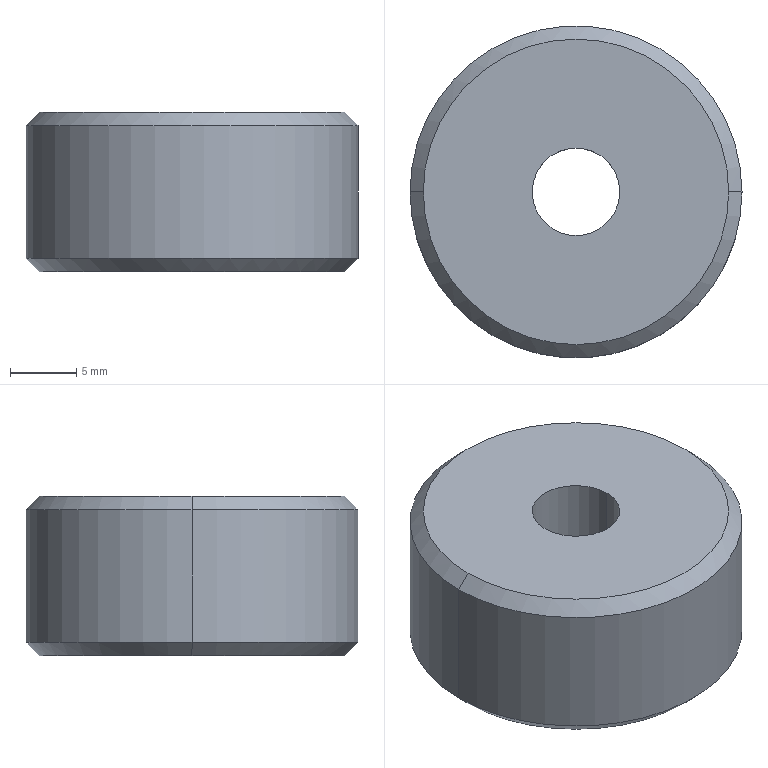Part | STEP file | 1 solid | 13 faces | box 25 x 25 x 12 mm | volume 5014 mm3 | cylinder 6 | cone 4 | plane 3 | commonest cylinder face diameters 6.6 x2 11 x2 25 x2
STEP:
#1=CARTESIAN_POINT('',(0.,0.,0.));
#2=DIRECTION('',(0.,0.,1.));
#3=DIRECTION('',(1.,0.,0.));
#4=AXIS2_PLACEMENT_3D('',#1,#2,#3);
#5=CARTESIAN_POINT('',(-11.5,0.,0.));
#6=VERTEX_POINT('',#5);
#7=CARTESIAN_POINT('',(11.5,0.,0.));
#8=VERTEX_POINT('',#7);
#9=CARTESIAN_POINT('',(0.,0.,0.));
#10=DIRECTION('',(0.,0.,-1.));
#11=DIRECTION('',(1.,0.,0.));
#12=AXIS2_PLACEMENT_3D('',#9,#10,#11);
#13=CIRCLE('',#12,11.5);
#14=CARTESIAN_POINT('',(0.,0.,1.));
#15=DIRECTION('',(0.,0.,1.));
#16=DIRECTION('',(1.,0.,0.));
#17=AXIS2_PLACEMENT_3D('',#14,#15,#16);
#18=CONICAL_SURFACE('',#17,12.5,0.7854);
#19=CARTESIAN_POINT('',(6.283,-1.));
#20=DIRECTION('',(-1.,0.));
#21=VECTOR('',#20,1.);
#22=LINE('',#19,#21);
#23=(GEOMETRIC_REPRESENTATION_CONTEXT(2)PARAMETRIC_REPRESENTATION_CONTEXT()REPRESENTATION_CONTEXT('',''));
#24=DEFINITIONAL_REPRESENTATION('',(#22),#23);
#25=PCURVE('',#18,#24);
#26=CARTESIAN_POINT('',(0.,0.,0.));
#27=DIRECTION('',(0.,0.,1.));
#28=DIRECTION('',(1.,0.,0.));
#29=AXIS2_PLACEMENT_3D('',#26,#27,#28);
#30=PLANE('',#29);
#31=CARTESIAN_POINT('',(11.5,0.));
#32=CARTESIAN_POINT('',(11.5,-19.919));
#33=CARTESIAN_POINT('',(-5.75,-9.959));
#34=CARTESIAN_POINT('',(-23.,0.));
#35=CARTESIAN_POINT('',(-5.75,9.959));
#36=CARTESIAN_POINT('',(11.5,19.919));
#37=CARTESIAN_POINT('',(11.5,0.));
#38=(BOUNDED_CURVE()B_SPLINE_CURVE(2,(#31,#32,#33,#34,#35,#36,#37),.UNSPECIFIED.,.T.,.F.)B_SPLINE_CURVE_WITH_KNOTS((1,2,2,2,2,1),(-2.094,0.,2.094,4.189,6.283,8.378),.UNSPECIFIED.)CURVE()GEOMETRIC_REPRESENTATION_ITEM()RATIONAL_B_SPLINE_CURVE((1.,0.5,1.,0.5,1.,0.5,1.))REPRESENTATION_ITEM(''));
#39=(GEOMETRIC_REPRESENTATION_CONTEXT(2)PARAMETRIC_REPRESENTATION_CONTEXT()REPRESENTATION_CONTEXT('',''));
#40=DEFINITIONAL_REPRESENTATION('',(#38),#39);
#41=PCURVE('',#30,#40);
#42=SURFACE_CURVE('',#13,(#25,#41),.PCURVE_S1.);
#43=EDGE_CURVE('',#6,#8,#42,.T.);
#44=ORIENTED_EDGE('',*,*,#43,.F.);
#45=CARTESIAN_POINT('',(-12.5,0.,1.));
#46=VERTEX_POINT('',#45);
#47=CARTESIAN_POINT('',(-12.5,0.,1.));
#48=DIRECTION('',(-0.7071,0.,0.7071));
#49=VECTOR('',#48,1.);
#50=LINE('',#47,#49);
#51=CARTESIAN_POINT('',(3.142,0.));
#52=DIRECTION('',(0.,1.));
#53=VECTOR('',#52,1.);
#54=LINE('',#51,#53);
#55=(GEOMETRIC_REPRESENTATION_CONTEXT(2)PARAMETRIC_REPRESENTATION_CONTEXT()REPRESENTATION_CONTEXT('',''));
#56=DEFINITIONAL_REPRESENTATION('',(#54),#55);
#57=PCURVE('',#18,#56);
#58=CARTESIAN_POINT('',(0.,0.,1.));
#59=DIRECTION('',(0.,0.,1.));
#60=DIRECTION('',(1.,0.,0.));
#61=AXIS2_PLACEMENT_3D('',#58,#59,#60);
#62=CONICAL_SURFACE('',#61,12.5,0.7854);
#63=CARTESIAN_POINT('',(3.142,0.));
#64=DIRECTION('',(0.,1.));
#65=VECTOR('',#64,1.);
#66=LINE('',#63,#65);
#67=(GEOMETRIC_REPRESENTATION_CONTEXT(2)PARAMETRIC_REPRESENTATION_CONTEXT()REPRESENTATION_CONTEXT('',''));
#68=DEFINITIONAL_REPRESENTATION('',(#66),#67);
#69=PCURVE('',#62,#68);
#70=SURFACE_CURVE('',#50,(#57,#69),.PCURVE_S1.);
#71=EDGE_CURVE('',#6,#46,#70,.T.);
#72=ORIENTED_EDGE('',*,*,#71,.T.);
#73=CARTESIAN_POINT('',(12.5,0.,1.));
#74=VERTEX_POINT('',#73);
#75=CARTESIAN_POINT('',(0.,0.,1.));
#76=DIRECTION('',(0.,0.,1.));
#77=DIRECTION('',(1.,0.,0.));
#78=AXIS2_PLACEMENT_3D('',#75,#76,#77);
#79=CIRCLE('',#78,12.5);
#80=CARTESIAN_POINT('',(0.,0.));
#81=DIRECTION('',(1.,0.));
#82=VECTOR('',#81,1.);
#83=LINE('',#80,#82);
#84=(GEOMETRIC_REPRESENTATION_CONTEXT(2)PARAMETRIC_REPRESENTATION_CONTEXT()REPRESENTATION_CONTEXT('',''));
#85=DEFINITIONAL_REPRESENTATION('',(#83),#84);
#86=PCURVE('',#18,#85);
#87=CARTESIAN_POINT('',(0.,0.,12.));
#88=DIRECTION('',(0.,0.,-1.));
#89=DIRECTION('',(-1.,0.,0.));
#90=AXIS2_PLACEMENT_3D('',#87,#88,#89);
#91=CYLINDRICAL_SURFACE('',#90,12.5);
#92=CARTESIAN_POINT('',(3.142,11.));
#93=DIRECTION('',(-1.,0.));
#94=VECTOR('',#93,1.);
#95=LINE('',#92,#94);
#96=(GEOMETRIC_REPRESENTATION_CONTEXT(2)PARAMETRIC_REPRESENTATION_CONTEXT()REPRESENTATION_CONTEXT('',''));
#97=DEFINITIONAL_REPRESENTATION('',(#95),#96);
#98=PCURVE('',#91,#97);
#99=SURFACE_CURVE('',#79,(#86,#98),.PCURVE_S1.);
#100=EDGE_CURVE('',#74,#46,#99,.T.);
#101=ORIENTED_EDGE('',*,*,#100,.F.);
#102=CARTESIAN_POINT('',(12.5,0.,1.));
#103=DIRECTION('',(0.7071,0.,0.7071));
#104=VECTOR('',#103,1.);
#105=LINE('',#102,#104);
#106=CARTESIAN_POINT('',(0.,0.));
#107=DIRECTION('',(0.,1.));
#108=VECTOR('',#107,1.);
#109=LINE('',#106,#108);
#110=(GEOMETRIC_REPRESENTATION_CONTEXT(2)PARAMETRIC_REPRESENTATION_CONTEXT()REPRESENTATION_CONTEXT('',''));
#111=DEFINITIONAL_REPRESENTATION('',(#109),#110);
#112=PCURVE('',#18,#111);
#113=CARTESIAN_POINT('',(6.283,0.));
#114=DIRECTION('',(0.,1.));
#115=VECTOR('',#114,1.);
#116=LINE('',#113,#115);
#117=(GEOMETRIC_REPRESENTATION_CONTEXT(2)PARAMETRIC_REPRESENTATION_CONTEXT()REPRESENTATION_CONTEXT('',''));
#118=DEFINITIONAL_REPRESENTATION('',(#116),#117);
#119=PCURVE('',#62,#118);
#120=SURFACE_CURVE('',#105,(#112,#119),.PCURVE_S1.);
#121=EDGE_CURVE('',#8,#74,#120,.T.);
#122=ORIENTED_EDGE('',*,*,#121,.F.);
#123=EDGE_LOOP('',(#44,#72,#101,#122));
#124=FACE_BOUND('',#123,.T.);
#125=ADVANCED_FACE('',(#124),#18,.T.);
#126=CARTESIAN_POINT('',(11.5,0.,12.));
#127=VERTEX_POINT('',#126);
#128=CARTESIAN_POINT('',(-11.5,0.,12.));
#129=VERTEX_POINT('',#128);
#130=CARTESIAN_POINT('',(0.,0.,12.));
#131=DIRECTION('',(0.,0.,1.));
#132=DIRECTION('',(1.,0.,0.));
#133=AXIS2_PLACEMENT_3D('',#130,#131,#132);
#134=CIRCLE('',#133,11.5);
#135=CARTESIAN_POINT('',(0.,0.,12.));
#136=DIRECTION('',(0.,0.,-1.));
#137=DIRECTION('',(-1.,0.,0.));
#138=AXIS2_PLACEMENT_3D('',#135,#136,#137);
#139=CONICAL_SURFACE('',#138,11.5,0.7854);
#140=CARTESIAN_POINT('',(3.142,0.));
#141=DIRECTION('',(-1.,0.));
#142=VECTOR('',#141,1.);
#143=LINE('',#140,#142);
#144=(GEOMETRIC_REPRESENTATION_CONTEXT(2)PARAMETRIC_REPRESENTATION_CONTEXT()REPRESENTATION_CONTEXT('',''));
#145=DEFINITIONAL_REPRESENTATION('',(#143),#144);
#146=PCURVE('',#139,#145);
#147=CARTESIAN_POINT('',(0.,0.,12.));
#148=DIRECTION('',(0.,0.,1.));
#149=DIRECTION('',(1.,0.,0.));
#150=AXIS2_PLACEMENT_3D('',#147,#148,#149);
#151=PLANE('',#150);
#152=CARTESIAN_POINT('',(0.,0.));
#153=DIRECTION('',(1.,0.));
#154=AXIS2_PLACEMENT_2D('',#152,#153);
#155=CIRCLE('',#154,11.5);
#156=(GEOMETRIC_REPRESENTATION_CONTEXT(2)PARAMETRIC_REPRESENTATION_CONTEXT()REPRESENTATION_CONTEXT('',''));
#157=DEFINITIONAL_REPRESENTATION('',(#155),#156);
#158=PCURVE('',#151,#157);
#159=SURFACE_CURVE('',#134,(#146,#158),.PCURVE_S1.);
#160=EDGE_CURVE('',#127,#129,#159,.T.);
#161=ORIENTED_EDGE('',*,*,#160,.F.);
#162=CARTESIAN_POINT('',(12.5,0.,11.));
#163=VERTEX_POINT('',#162);
#164=CARTESIAN_POINT('',(11.5,0.,12.));
#165=DIRECTION('',(0.7071,0.,-0.7071));
#166=VECTOR('',#165,1.);
#167=LINE('',#164,#166);
#168=CARTESIAN_POINT('',(3.142,0.));
#169=DIRECTION('',(0.,1.));
#170=VECTOR('',#169,1.);
#171=LINE('',#168,#170);
#172=(GEOMETRIC_REPRESENTATION_CONTEXT(2)PARAMETRIC_REPRESENTATION_CONTEXT()REPRESENTATION_CONTEXT('',''));
#173=DEFINITIONAL_REPRESENTATION('',(#171),#172);
#174=PCURVE('',#139,#173);
#175=CARTESIAN_POINT('',(0.,0.,12.));
#176=DIRECTION('',(0.,0.,-1.));
#177=DIRECTION('',(-1.,0.,0.));
#178=AXIS2_PLACEMENT_3D('',#175,#176,#177);
#179=CONICAL_SURFACE('',#178,11.5,0.7854);
#180=CARTESIAN_POINT('',(3.142,0.));
#181=DIRECTION('',(0.,1.));
#182=VECTOR('',#181,1.);
#183=LINE('',#180,#182);
#184=(GEOMETRIC_REPRESENTATION_CONTEXT(2)PARAMETRIC_REPRESENTATION_CONTEXT()REPRESENTATION_CONTEXT('',''));
#185=DEFINITIONAL_REPRESENTATION('',(#183),#184);
#186=PCURVE('',#179,#185);
#187=SURFACE_CURVE('',#167,(#174,#186),.PCURVE_S1.);
#188=EDGE_CURVE('',#127,#163,#187,.T.);
#189=ORIENTED_EDGE('',*,*,#188,.T.);
#190=CARTESIAN_POINT('',(-12.5,0.,11.));
#191=VERTEX_POINT('',#190);
#192=CARTESIAN_POINT('',(0.,0.,11.));
#193=DIRECTION('',(0.,0.,-1.));
#194=DIRECTION('',(1.,0.,0.));
#195=AXIS2_PLACEMENT_3D('',#192,#193,#194);
#196=CIRCLE('',#195,12.5);
#197=CARTESIAN_POINT('',(-3.142,1.));
#198=DIRECTION('',(1.,0.));
#199=VECTOR('',#198,1.);
#200=LINE('',#197,#199);
#201=(GEOMETRIC_REPRESENTATION_CONTEXT(2)PARAMETRIC_REPRESENTATION_CONTEXT()REPRESENTATION_CONTEXT('',''));
#202=DEFINITIONAL_REPRESENTATION('',(#200),#201);
#203=PCURVE('',#139,#202);
#204=CARTESIAN_POINT('',(-3.142,1.));
#205=DIRECTION('',(1.,0.));
#206=VECTOR('',#205,1.);
#207=LINE('',#204,#206);
#208=(GEOMETRIC_REPRESENTATION_CONTEXT(2)PARAMETRIC_REPRESENTATION_CONTEXT()REPRESENTATION_CONTEXT('',''));
#209=DEFINITIONAL_REPRESENTATION('',(#207),#208);
#210=PCURVE('',#91,#209);
#211=SURFACE_CURVE('',#196,(#203,#210),.PCURVE_S1.);
#212=EDGE_CURVE('',#191,#163,#211,.T.);
#213=ORIENTED_EDGE('',*,*,#212,.F.);
#214=CARTESIAN_POINT('',(-11.5,0.,12.));
#215=DIRECTION('',(-0.7071,0.,-0.7071));
#216=VECTOR('',#215,1.);
#217=LINE('',#214,#216);
#218=CARTESIAN_POINT('',(0.,0.));
#219=DIRECTION('',(0.,1.));
#220=VECTOR('',#219,1.);
#221=LINE('',#218,#220);
#222=(GEOMETRIC_REPRESENTATION_CONTEXT(2)PARAMETRIC_REPRESENTATION_CONTEXT()REPRESENTATION_CONTEXT('',''));
#223=DEFINITIONAL_REPRESENTATION('',(#221),#222);
#224=PCURVE('',#139,#223);
#225=CARTESIAN_POINT('',(6.283,0.));
#226=DIRECTION('',(0.,1.));
#227=VECTOR('',#226,1.);
#228=LINE('',#225,#227);
#229=(GEOMETRIC_REPRESENTATION_CONTEXT(2)PARAMETRIC_REPRESENTATION_CONTEXT()REPRESENTATION_CONTEXT('',''));
#230=DEFINITIONAL_REPRESENTATION('',(#228),#229);
#231=PCURVE('',#179,#230);
#232=SURFACE_CURVE('',#217,(#224,#231),.PCURVE_S1.);
#233=EDGE_CURVE('',#129,#191,#232,.T.);
#234=ORIENTED_EDGE('',*,*,#233,.F.);
#235=EDGE_LOOP('',(#161,#189,#213,#234));
#236=FACE_BOUND('',#235,.T.);
#237=ADVANCED_FACE('',(#236),#139,.T.);
#238=CARTESIAN_POINT('',(-5.5,0.,6.4));
#239=VERTEX_POINT('',#238);
#240=CARTESIAN_POINT('',(-5.5,0.,0.));
#241=VERTEX_POINT('',#240);
#242=CARTESIAN_POINT('',(-5.5,0.,0.));
#243=DIRECTION('',(0.,0.,-1.));
#244=VECTOR('',#243,1.);
#245=LINE('',#242,#244);
#246=CARTESIAN_POINT('',(0.,0.,0.));
#247=DIRECTION('',(0.,0.,-1.));
#248=DIRECTION('',(-1.,0.,0.));
#249=AXIS2_PLACEMENT_3D('',#246,#247,#248);
#250=CYLINDRICAL_SURFACE('',#249,5.5);
#251=CARTESIAN_POINT('',(6.283,0.));
#252=DIRECTION('',(0.,1.));
#253=VECTOR('',#252,1.);
#254=LINE('',#251,#253);
#255=(GEOMETRIC_REPRESENTATION_CONTEXT(2)PARAMETRIC_REPRESENTATION_CONTEXT()REPRESENTATION_CONTEXT('',''));
#256=DEFINITIONAL_REPRESENTATION('',(#254),#255);
#257=PCURVE('',#250,#256);
#258=CARTESIAN_POINT('',(0.,0.,0.));
#259=DIRECTION('',(0.,0.,-1.));
#260=DIRECTION('',(-1.,0.,0.));
#261=AXIS2_PLACEMENT_3D('',#258,#259,#260);
#262=CYLINDRICAL_SURFACE('',#261,5.5);
#263=CARTESIAN_POINT('',(0.,0.));
#264=DIRECTION('',(0.,1.));
#265=VECTOR('',#264,1.);
#266=LINE('',#263,#265);
#267=(GEOMETRIC_REPRESENTATION_CONTEXT(2)PARAMETRIC_REPRESENTATION_CONTEXT()REPRESENTATION_CONTEXT('',''));
#268=DEFINITIONAL_REPRESENTATION('',(#266),#267);
#269=PCURVE('',#262,#268);
#270=SURFACE_CURVE('',#245,(#257,#269),.PCURVE_S1.);
#271=EDGE_CURVE('',#239,#241,#270,.T.);
#272=ORIENTED_EDGE('',*,*,#271,.T.);
#273=CARTESIAN_POINT('',(5.5,0.,0.));
#274=VERTEX_POINT('',#273);
#275=CARTESIAN_POINT('',(0.,0.,0.));
#276=DIRECTION('',(0.,0.,-1.));
#277=DIRECTION('',(-1.,0.,0.));
#278=AXIS2_PLACEMENT_3D('',#275,#276,#277);
#279=CIRCLE('',#278,5.5);
#280=CARTESIAN_POINT('',(0.,0.));
#281=DIRECTION('',(1.,0.));
#282=VECTOR('',#281,1.);
#283=LINE('',#280,#282);
#284=(GEOMETRIC_REPRESENTATION_CONTEXT(2)PARAMETRIC_REPRESENTATION_CONTEXT()REPRESENTATION_CONTEXT('',''));
#285=DEFINITIONAL_REPRESENTATION('',(#283),#284);
#286=PCURVE('',#250,#285);
#287=CARTESIAN_POINT('',(-5.5,0.));
#288=CARTESIAN_POINT('',(-5.5,9.526));
#289=CARTESIAN_POINT('',(2.75,4.763));
#290=CARTESIAN_POINT('',(11.,0.));
#291=CARTESIAN_POINT('',(2.75,-4.763));
#292=CARTESIAN_POINT('',(-5.5,-9.526));
#293=CARTESIAN_POINT('',(-5.5,0.));
#294=(BOUNDED_CURVE()B_SPLINE_CURVE(2,(#287,#288,#289,#290,#291,#292,#293),.UNSPECIFIED.,.T.,.F.)B_SPLINE_CURVE_WITH_KNOTS((1,2,2,2,2,1),(-2.094,0.,2.094,4.189,6.283,8.378),.UNSPECIFIED.)CURVE()GEOMETRIC_REPRESENTATION_ITEM()RATIONAL_B_SPLINE_CURVE((1.,0.5,1.,0.5,1.,0.5,1.))REPRESENTATION_ITEM(''));
#295=(GEOMETRIC_REPRESENTATION_CONTEXT(2)PARAMETRIC_REPRESENTATION_CONTEXT()REPRESENTATION_CONTEXT('',''));
#296=DEFINITIONAL_REPRESENTATION('',(#294),#295);
#297=PCURVE('',#30,#296);
#298=SURFACE_CURVE('',#279,(#286,#297),.PCURVE_S1.);
#299=EDGE_CURVE('',#274,#241,#298,.T.);
#300=ORIENTED_EDGE('',*,*,#299,.F.);
#301=CARTESIAN_POINT('',(5.5,0.,6.4));
#302=VERTEX_POINT('',#301);
#303=CARTESIAN_POINT('',(5.5,0.,0.));
#304=DIRECTION('',(0.,0.,-1.));
#305=VECTOR('',#304,1.);
#306=LINE('',#303,#305);
#307=CARTESIAN_POINT('',(3.142,0.));
#308=DIRECTION('',(0.,1.));
#309=VECTOR('',#308,1.);
#310=LINE('',#307,#309);
#311=(GEOMETRIC_REPRESENTATION_CONTEXT(2)PARAMETRIC_REPRESENTATION_CONTEXT()REPRESENTATION_CONTEXT('',''));
#312=DEFINITIONAL_REPRESENTATION('',(#310),#311);
#313=PCURVE('',#250,#312);
#314=CARTESIAN_POINT('',(3.142,0.));
#315=DIRECTION('',(0.,1.));
#316=VECTOR('',#315,1.);
#317=LINE('',#314,#316);
#318=(GEOMETRIC_REPRESENTATION_CONTEXT(2)PARAMETRIC_REPRESENTATION_CONTEXT()REPRESENTATION_CONTEXT('',''));
#319=DEFINITIONAL_REPRESENTATION('',(#317),#318);
#320=PCURVE('',#262,#319);
#321=SURFACE_CURVE('',#306,(#313,#320),.PCURVE_S1.);
#322=EDGE_CURVE('',#302,#274,#321,.T.);
#323=ORIENTED_EDGE('',*,*,#322,.F.);
#324=CARTESIAN_POINT('',(0.,0.,6.4));
#325=DIRECTION('',(0.,0.,-1.));
#326=DIRECTION('',(-1.,0.,0.));
#327=AXIS2_PLACEMENT_3D('',#324,#325,#326);
#328=CIRCLE('',#327,5.5);
#329=CARTESIAN_POINT('',(0.,-6.4));
#330=DIRECTION('',(1.,0.));
#331=VECTOR('',#330,1.);
#332=LINE('',#329,#331);
#333=(GEOMETRIC_REPRESENTATION_CONTEXT(2)PARAMETRIC_REPRESENTATION_CONTEXT()REPRESENTATION_CONTEXT('',''));
#334=DEFINITIONAL_REPRESENTATION('',(#332),#333);
#335=PCURVE('',#250,#334);
#336=CARTESIAN_POINT('',(3.3,0.,6.4));
#337=DIRECTION('',(0.,0.,1.));
#338=DIRECTION('',(1.,0.,0.));
#339=AXIS2_PLACEMENT_3D('',#336,#337,#338);
#340=PLANE('',#339);
#341=CARTESIAN_POINT('',(-8.8,0.));
#342=CARTESIAN_POINT('',(-8.8,9.526));
#343=CARTESIAN_POINT('',(-0.55,4.763));
#344=CARTESIAN_POINT('',(7.7,0.));
#345=CARTESIAN_POINT('',(-0.55,-4.763));
#346=CARTESIAN_POINT('',(-8.8,-9.526));
#347=CARTESIAN_POINT('',(-8.8,0.));
#348=(BOUNDED_CURVE()B_SPLINE_CURVE(2,(#341,#342,#343,#344,#345,#346,#347),.UNSPECIFIED.,.T.,.F.)B_SPLINE_CURVE_WITH_KNOTS((1,2,2,2,2,1),(-2.094,0.,2.094,4.189,6.283,8.378),.UNSPECIFIED.)CURVE()GEOMETRIC_REPRESENTATION_ITEM()RATIONAL_B_SPLINE_CURVE((1.,0.5,1.,0.5,1.,0.5,1.))REPRESENTATION_ITEM(''));
#349=(GEOMETRIC_REPRESENTATION_CONTEXT(2)PARAMETRIC_REPRESENTATION_CONTEXT()REPRESENTATION_CONTEXT('',''));
#350=DEFINITIONAL_REPRESENTATION('',(#348),#349);
#351=PCURVE('',#340,#350);
#352=SURFACE_CURVE('',#328,(#335,#351),.PCURVE_S1.);
#353=EDGE_CURVE('',#302,#239,#352,.T.);
#354=ORIENTED_EDGE('',*,*,#353,.T.);
#355=EDGE_LOOP('',(#272,#300,#323,#354));
#356=FACE_BOUND('',#355,.F.);
#357=ADVANCED_FACE('',(#356),#250,.F.);
#358=CARTESIAN_POINT('',(-3.3,0.,12.));
#359=VERTEX_POINT('',#358);
#360=CARTESIAN_POINT('',(-3.3,0.,6.4));
#361=VERTEX_POINT('',#360);
#362=CARTESIAN_POINT('',(-3.3,0.,0.));
#363=DIRECTION('',(0.,0.,-1.));
#364=VECTOR('',#363,1.);
#365=LINE('',#362,#364);
#366=CARTESIAN_POINT('',(0.,0.,0.));
#367=DIRECTION('',(0.,0.,-1.));
#368=DIRECTION('',(-1.,0.,0.));
#369=AXIS2_PLACEMENT_3D('',#366,#367,#368);
#370=CYLINDRICAL_SURFACE('',#369,3.3);
#371=CARTESIAN_POINT('',(6.283,0.));
#372=DIRECTION('',(0.,1.));
#373=VECTOR('',#372,1.);
#374=LINE('',#371,#373);
#375=(GEOMETRIC_REPRESENTATION_CONTEXT(2)PARAMETRIC_REPRESENTATION_CONTEXT()REPRESENTATION_CONTEXT('',''));
#376=DEFINITIONAL_REPRESENTATION('',(#374),#375);
#377=PCURVE('',#370,#376);
#378=CARTESIAN_POINT('',(0.,0.,0.));
#379=DIRECTION('',(0.,0.,-1.));
#380=DIRECTION('',(-1.,0.,0.));
#381=AXIS2_PLACEMENT_3D('',#378,#379,#380);
#382=CYLINDRICAL_SURFACE('',#381,3.3);
#383=CARTESIAN_POINT('',(0.,0.));
#384=DIRECTION('',(0.,1.));
#385=VECTOR('',#384,1.);
#386=LINE('',#383,#385);
#387=(GEOMETRIC_REPRESENTATION_CONTEXT(2)PARAMETRIC_REPRESENTATION_CONTEXT()REPRESENTATION_CONTEXT('',''));
#388=DEFINITIONAL_REPRESENTATION('',(#386),#387);
#389=PCURVE('',#382,#388);
#390=SURFACE_CURVE('',#365,(#377,#389),.PCURVE_S1.);
#391=EDGE_CURVE('',#359,#361,#390,.T.);
#392=ORIENTED_EDGE('',*,*,#391,.T.);
#393=CARTESIAN_POINT('',(3.3,0.,6.4));
#394=VERTEX_POINT('',#393);
#395=CARTESIAN_POINT('',(0.,0.,6.4));
#396=DIRECTION('',(0.,0.,-1.));
#397=DIRECTION('',(-1.,0.,0.));
#398=AXIS2_PLACEMENT_3D('',#395,#396,#397);
#399=CIRCLE('',#398,3.3);
#400=CARTESIAN_POINT('',(0.,-6.4));
#401=DIRECTION('',(1.,0.));
#402=VECTOR('',#401,1.);
#403=LINE('',#400,#402);
#404=(GEOMETRIC_REPRESENTATION_CONTEXT(2)PARAMETRIC_REPRESENTATION_CONTEXT()REPRESENTATION_CONTEXT('',''));
#405=DEFINITIONAL_REPRESENTATION('',(#403),#404);
#406=PCURVE('',#370,#405);
#407=CARTESIAN_POINT('',(-6.6,0.));
#408=CARTESIAN_POINT('',(-6.6,5.716));
#409=CARTESIAN_POINT('',(-1.65,2.858));
#410=CARTESIAN_POINT('',(3.3,0.));
#411=CARTESIAN_POINT('',(-1.65,-2.858));
#412=CARTESIAN_POINT('',(-6.6,-5.716));
#413=CARTESIAN_POINT('',(-6.6,0.));
#414=(BOUNDED_CURVE()B_SPLINE_CURVE(2,(#407,#408,#409,#410,#411,#412,#413),.UNSPECIFIED.,.T.,.F.)B_SPLINE_CURVE_WITH_KNOTS((1,2,2,2,2,1),(-2.094,0.,2.094,4.189,6.283,8.378),.UNSPECIFIED.)CURVE()GEOMETRIC_REPRESENTATION_ITEM()RATIONAL_B_SPLINE_CURVE((1.,0.5,1.,0.5,1.,0.5,1.))REPRESENTATION_ITEM(''));
#415=(GEOMETRIC_REPRESENTATION_CONTEXT(2)PARAMETRIC_REPRESENTATION_CONTEXT()REPRESENTATION_CONTEXT('',''));
#416=DEFINITIONAL_REPRESENTATION('',(#414),#415);
#417=PCURVE('',#340,#416);
#418=SURFACE_CURVE('',#399,(#406,#417),.PCURVE_S1.);
#419=EDGE_CURVE('',#394,#361,#418,.T.);
#420=ORIENTED_EDGE('',*,*,#419,.F.);
#421=CARTESIAN_POINT('',(3.3,0.,12.));
#422=VERTEX_POINT('',#421);
#423=CARTESIAN_POINT('',(3.3,0.,0.));
#424=DIRECTION('',(0.,0.,-1.));
#425=VECTOR('',#424,1.);
#426=LINE('',#423,#425);
#427=CARTESIAN_POINT('',(3.142,0.));
#428=DIRECTION('',(0.,1.));
#429=VECTOR('',#428,1.);
#430=LINE('',#427,#429);
#431=(GEOMETRIC_REPRESENTATION_CONTEXT(2)PARAMETRIC_REPRESENTATION_CONTEXT()REPRESENTATION_CONTEXT('',''));
#432=DEFINITIONAL_REPRESENTATION('',(#430),#431);
#433=PCURVE('',#370,#432);
#434=CARTESIAN_POINT('',(3.142,0.));
#435=DIRECTION('',(0.,1.));
#436=VECTOR('',#435,1.);
#437=LINE('',#434,#436);
#438=(GEOMETRIC_REPRESENTATION_CONTEXT(2)PARAMETRIC_REPRESENTATION_CONTEXT()REPRESENTATION_CONTEXT('',''));
#439=DEFINITIONAL_REPRESENTATION('',(#437),#438);
#440=PCURVE('',#382,#439);
#441=SURFACE_CURVE('',#426,(#433,#440),.PCURVE_S1.);
#442=EDGE_CURVE('',#422,#394,#441,.T.);
#443=ORIENTED_EDGE('',*,*,#442,.F.);
#444=CARTESIAN_POINT('',(0.,0.,12.));
#445=DIRECTION('',(0.,0.,-1.));
#446=DIRECTION('',(-1.,0.,0.));
#447=AXIS2_PLACEMENT_3D('',#444,#445,#446);
#448=CIRCLE('',#447,3.3);
#449=CARTESIAN_POINT('',(0.,-12.));
#450=DIRECTION('',(1.,0.));
#451=VECTOR('',#450,1.);
#452=LINE('',#449,#451);
#453=(GEOMETRIC_REPRESENTATION_CONTEXT(2)PARAMETRIC_REPRESENTATION_CONTEXT()REPRESENTATION_CONTEXT('',''));
#454=DEFINITIONAL_REPRESENTATION('',(#452),#453);
#455=PCURVE('',#370,#454);
#456=CARTESIAN_POINT('',(-3.3,0.));
#457=CARTESIAN_POINT('',(-3.3,5.716));
#458=CARTESIAN_POINT('',(1.65,2.858));
#459=CARTESIAN_POINT('',(6.6,0.));
#460=CARTESIAN_POINT('',(1.65,-2.858));
#461=CARTESIAN_POINT('',(-3.3,-5.716));
#462=CARTESIAN_POINT('',(-3.3,0.));
#463=(BOUNDED_CURVE()B_SPLINE_CURVE(2,(#456,#457,#458,#459,#460,#461,#462),.UNSPECIFIED.,.T.,.F.)B_SPLINE_CURVE_WITH_KNOTS((1,2,2,2,2,1),(-2.094,0.,2.094,4.189,6.283,8.378),.UNSPECIFIED.)CURVE()GEOMETRIC_REPRESENTATION_ITEM()RATIONAL_B_SPLINE_CURVE((1.,0.5,1.,0.5,1.,0.5,1.))REPRESENTATION_ITEM(''));
#464=(GEOMETRIC_REPRESENTATION_CONTEXT(2)PARAMETRIC_REPRESENTATION_CONTEXT()REPRESENTATION_CONTEXT('',''));
#465=DEFINITIONAL_REPRESENTATION('',(#463),#464);
#466=PCURVE('',#151,#465);
#467=SURFACE_CURVE('',#448,(#455,#466),.PCURVE_S1.);
#468=EDGE_CURVE('',#422,#359,#467,.T.);
#469=ORIENTED_EDGE('',*,*,#468,.T.);
#470=EDGE_LOOP('',(#392,#420,#443,#469));
#471=FACE_BOUND('',#470,.F.);
#472=ADVANCED_FACE('',(#471),#370,.F.);
#473=ORIENTED_EDGE('',*,*,#212,.T.);
#474=CARTESIAN_POINT('',(12.5,0.,12.));
#475=DIRECTION('',(0.,0.,-1.));
#476=VECTOR('',#475,1.);
#477=LINE('',#474,#476);
#478=CARTESIAN_POINT('',(3.142,0.));
#479=DIRECTION('',(0.,1.));
#480=VECTOR('',#479,1.);
#481=LINE('',#478,#480);
#482=(GEOMETRIC_REPRESENTATION_CONTEXT(2)PARAMETRIC_REPRESENTATION_CONTEXT()REPRESENTATION_CONTEXT('',''));
#483=DEFINITIONAL_REPRESENTATION('',(#481),#482);
#484=PCURVE('',#91,#483);
#485=CARTESIAN_POINT('',(0.,0.,12.));
#486=DIRECTION('',(0.,0.,-1.));
#487=DIRECTION('',(-1.,0.,0.));
#488=AXIS2_PLACEMENT_3D('',#485,#486,#487);
#489=CYLINDRICAL_SURFACE('',#488,12.5);
#490=CARTESIAN_POINT('',(3.142,0.));
#491=DIRECTION('',(0.,1.));
#492=VECTOR('',#491,1.);
#493=LINE('',#490,#492);
#494=(GEOMETRIC_REPRESENTATION_CONTEXT(2)PARAMETRIC_REPRESENTATION_CONTEXT()REPRESENTATION_CONTEXT('',''));
#495=DEFINITIONAL_REPRESENTATION('',(#493),#494);
#496=PCURVE('',#489,#495);
#497=SURFACE_CURVE('',#477,(#484,#496),.PCURVE_S1.);
#498=EDGE_CURVE('',#163,#74,#497,.T.);
#499=ORIENTED_EDGE('',*,*,#498,.T.);
#500=ORIENTED_EDGE('',*,*,#100,.T.);
#501=CARTESIAN_POINT('',(-12.5,0.,12.));
#502=DIRECTION('',(0.,0.,-1.));
#503=VECTOR('',#502,1.);
#504=LINE('',#501,#503);
#505=CARTESIAN_POINT('',(0.,0.));
#506=DIRECTION('',(0.,1.));
#507=VECTOR('',#506,1.);
#508=LINE('',#505,#507);
#509=(GEOMETRIC_REPRESENTATION_CONTEXT(2)PARAMETRIC_REPRESENTATION_CONTEXT()REPRESENTATION_CONTEXT('',''));
#510=DEFINITIONAL_REPRESENTATION('',(#508),#509);
#511=PCURVE('',#91,#510);
#512=CARTESIAN_POINT('',(6.283,0.));
#513=DIRECTION('',(0.,1.));
#514=VECTOR('',#513,1.);
#515=LINE('',#512,#514);
#516=(GEOMETRIC_REPRESENTATION_CONTEXT(2)PARAMETRIC_REPRESENTATION_CONTEXT()REPRESENTATION_CONTEXT('',''));
#517=DEFINITIONAL_REPRESENTATION('',(#515),#516);
#518=PCURVE('',#489,#517);
#519=SURFACE_CURVE('',#504,(#511,#518),.PCURVE_S1.);
#520=EDGE_CURVE('',#191,#46,#519,.T.);
#521=ORIENTED_EDGE('',*,*,#520,.F.);
#522=EDGE_LOOP('',(#473,#499,#500,#521));
#523=FACE_BOUND('',#522,.T.);
#524=ADVANCED_FACE('',(#523),#91,.T.);
#525=ORIENTED_EDGE('',*,*,#498,.F.);
#526=CARTESIAN_POINT('',(0.,0.,11.));
#527=DIRECTION('',(0.,0.,-1.));
#528=DIRECTION('',(1.,0.,0.));
#529=AXIS2_PLACEMENT_3D('',#526,#527,#528);
#530=CIRCLE('',#529,12.5);
#531=CARTESIAN_POINT('',(3.142,1.));
#532=DIRECTION('',(1.,0.));
#533=VECTOR('',#532,1.);
#534=LINE('',#531,#533);
#535=(GEOMETRIC_REPRESENTATION_CONTEXT(2)PARAMETRIC_REPRESENTATION_CONTEXT()REPRESENTATION_CONTEXT('',''));
#536=DEFINITIONAL_REPRESENTATION('',(#534),#535);
#537=PCURVE('',#489,#536);
#538=CARTESIAN_POINT('',(3.142,1.));
#539=DIRECTION('',(1.,0.));
#540=VECTOR('',#539,1.);
#541=LINE('',#538,#540);
#542=(GEOMETRIC_REPRESENTATION_CONTEXT(2)PARAMETRIC_REPRESENTATION_CONTEXT()REPRESENTATION_CONTEXT('',''));
#543=DEFINITIONAL_REPRESENTATION('',(#541),#542);
#544=PCURVE('',#179,#543);
#545=SURFACE_CURVE('',#530,(#537,#544),.PCURVE_S1.);
#546=EDGE_CURVE('',#163,#191,#545,.T.);
#547=ORIENTED_EDGE('',*,*,#546,.T.);
#548=ORIENTED_EDGE('',*,*,#520,.T.);
#549=CARTESIAN_POINT('',(0.,0.,1.));
#550=DIRECTION('',(0.,0.,1.));
#551=DIRECTION('',(1.,0.,0.));
#552=AXIS2_PLACEMENT_3D('',#549,#550,#551);
#553=CIRCLE('',#552,12.5);
#554=CARTESIAN_POINT('',(9.425,11.));
#555=DIRECTION('',(-1.,0.));
#556=VECTOR('',#555,1.);
#557=LINE('',#554,#556);
#558=(GEOMETRIC_REPRESENTATION_CONTEXT(2)PARAMETRIC_REPRESENTATION_CONTEXT()REPRESENTATION_CONTEXT('',''));
#559=DEFINITIONAL_REPRESENTATION('',(#557),#558);
#560=PCURVE('',#489,#559);
#561=CARTESIAN_POINT('',(0.,0.));
#562=DIRECTION('',(1.,0.));
#563=VECTOR('',#562,1.);
#564=LINE('',#561,#563);
#565=(GEOMETRIC_REPRESENTATION_CONTEXT(2)PARAMETRIC_REPRESENTATION_CONTEXT()REPRESENTATION_CONTEXT('',''));
#566=DEFINITIONAL_REPRESENTATION('',(#564),#565);
#567=PCURVE('',#62,#566);
#568=SURFACE_CURVE('',#553,(#560,#567),.PCURVE_S1.);
#569=EDGE_CURVE('',#46,#74,#568,.T.);
#570=ORIENTED_EDGE('',*,*,#569,.T.);
#571=EDGE_LOOP('',(#525,#547,#548,#570));
#572=FACE_BOUND('',#571,.T.);
#573=ADVANCED_FACE('',(#572),#489,.T.);
#574=CARTESIAN_POINT('',(0.,0.,12.));
#575=DIRECTION('',(0.,0.,1.));
#576=DIRECTION('',(1.,0.,0.));
#577=AXIS2_PLACEMENT_3D('',#574,#575,#576);
#578=CIRCLE('',#577,11.5);
#579=CARTESIAN_POINT('',(0.,0.));
#580=DIRECTION('',(1.,0.));
#581=AXIS2_PLACEMENT_2D('',#579,#580);
#582=CIRCLE('',#581,11.5);
#583=(GEOMETRIC_REPRESENTATION_CONTEXT(2)PARAMETRIC_REPRESENTATION_CONTEXT()REPRESENTATION_CONTEXT('',''));
#584=DEFINITIONAL_REPRESENTATION('',(#582),#583);
#585=PCURVE('',#151,#584);
#586=CARTESIAN_POINT('',(9.425,0.));
#587=DIRECTION('',(-1.,0.));
#588=VECTOR('',#587,1.);
#589=LINE('',#586,#588);
#590=(GEOMETRIC_REPRESENTATION_CONTEXT(2)PARAMETRIC_REPRESENTATION_CONTEXT()REPRESENTATION_CONTEXT('',''));
#591=DEFINITIONAL_REPRESENTATION('',(#589),#590);
#592=PCURVE('',#179,#591);
#593=SURFACE_CURVE('',#578,(#585,#592),.PCURVE_S1.);
#594=EDGE_CURVE('',#129,#127,#593,.T.);
#595=ORIENTED_EDGE('',*,*,#594,.T.);
#596=ORIENTED_EDGE('',*,*,#160,.T.);
#597=EDGE_LOOP('',(#595,#596));
#598=FACE_BOUND('',#597,.T.);
#599=CARTESIAN_POINT('',(0.,0.,12.));
#600=DIRECTION('',(0.,0.,-1.));
#601=DIRECTION('',(-1.,0.,0.));
#602=AXIS2_PLACEMENT_3D('',#599,#600,#601);
#603=CIRCLE('',#602,3.3);
#604=CARTESIAN_POINT('',(-3.3,0.));
#605=CARTESIAN_POINT('',(-3.3,5.716));
#606=CARTESIAN_POINT('',(1.65,2.858));
#607=CARTESIAN_POINT('',(6.6,0.));
#608=CARTESIAN_POINT('',(1.65,-2.858));
#609=CARTESIAN_POINT('',(-3.3,-5.716));
#610=CARTESIAN_POINT('',(-3.3,0.));
#611=(BOUNDED_CURVE()B_SPLINE_CURVE(2,(#604,#605,#606,#607,#608,#609,#610),.UNSPECIFIED.,.T.,.F.)B_SPLINE_CURVE_WITH_KNOTS((1,2,2,2,2,1),(-2.094,0.,2.094,4.189,6.283,8.378),.UNSPECIFIED.)CURVE()GEOMETRIC_REPRESENTATION_ITEM()RATIONAL_B_SPLINE_CURVE((1.,0.5,1.,0.5,1.,0.5,1.))REPRESENTATION_ITEM(''));
#612=(GEOMETRIC_REPRESENTATION_CONTEXT(2)PARAMETRIC_REPRESENTATION_CONTEXT()REPRESENTATION_CONTEXT('',''));
#613=DEFINITIONAL_REPRESENTATION('',(#611),#612);
#614=PCURVE('',#151,#613);
#615=CARTESIAN_POINT('',(0.,-12.));
#616=DIRECTION('',(1.,0.));
#617=VECTOR('',#616,1.);
#618=LINE('',#615,#617);
#619=(GEOMETRIC_REPRESENTATION_CONTEXT(2)PARAMETRIC_REPRESENTATION_CONTEXT()REPRESENTATION_CONTEXT('',''));
#620=DEFINITIONAL_REPRESENTATION('',(#618),#619);
#621=PCURVE('',#382,#620);
#622=SURFACE_CURVE('',#603,(#614,#621),.PCURVE_S1.);
#623=EDGE_CURVE('',#359,#422,#622,.T.);
#624=ORIENTED_EDGE('',*,*,#623,.T.);
#625=ORIENTED_EDGE('',*,*,#468,.T.);
#626=EDGE_LOOP('',(#624,#625));
#627=FACE_BOUND('',#626,.T.);
#628=ADVANCED_FACE('',(#598,#627),#151,.T.);
#629=CARTESIAN_POINT('',(0.,0.,0.));
#630=DIRECTION('',(0.,0.,-1.));
#631=DIRECTION('',(1.,0.,0.));
#632=AXIS2_PLACEMENT_3D('',#629,#630,#631);
#633=CIRCLE('',#632,11.5);
#634=CARTESIAN_POINT('',(11.5,0.));
#635=CARTESIAN_POINT('',(11.5,-19.919));
#636=CARTESIAN_POINT('',(-5.75,-9.959));
#637=CARTESIAN_POINT('',(-23.,0.));
#638=CARTESIAN_POINT('',(-5.75,9.959));
#639=CARTESIAN_POINT('',(11.5,19.919));
#640=CARTESIAN_POINT('',(11.5,0.));
#641=(BOUNDED_CURVE()B_SPLINE_CURVE(2,(#634,#635,#636,#637,#638,#639,#640),.UNSPECIFIED.,.T.,.F.)B_SPLINE_CURVE_WITH_KNOTS((1,2,2,2,2,1),(-2.094,0.,2.094,4.189,6.283,8.378),.UNSPECIFIED.)CURVE()GEOMETRIC_REPRESENTATION_ITEM()RATIONAL_B_SPLINE_CURVE((1.,0.5,1.,0.5,1.,0.5,1.))REPRESENTATION_ITEM(''));
#642=(GEOMETRIC_REPRESENTATION_CONTEXT(2)PARAMETRIC_REPRESENTATION_CONTEXT()REPRESENTATION_CONTEXT('',''));
#643=DEFINITIONAL_REPRESENTATION('',(#641),#642);
#644=PCURVE('',#30,#643);
#645=CARTESIAN_POINT('',(6.283,-1.));
#646=DIRECTION('',(-1.,0.));
#647=VECTOR('',#646,1.);
#648=LINE('',#645,#647);
#649=(GEOMETRIC_REPRESENTATION_CONTEXT(2)PARAMETRIC_REPRESENTATION_CONTEXT()REPRESENTATION_CONTEXT('',''));
#650=DEFINITIONAL_REPRESENTATION('',(#648),#649);
#651=PCURVE('',#62,#650);
#652=SURFACE_CURVE('',#633,(#644,#651),.PCURVE_S1.);
#653=EDGE_CURVE('',#8,#6,#652,.T.);
#654=ORIENTED_EDGE('',*,*,#653,.T.);
#655=ORIENTED_EDGE('',*,*,#43,.T.);
#656=EDGE_LOOP('',(#654,#655));
#657=FACE_BOUND('',#656,.T.);
#658=CARTESIAN_POINT('',(0.,0.,0.));
#659=DIRECTION('',(0.,0.,-1.));
#660=DIRECTION('',(-1.,0.,0.));
#661=AXIS2_PLACEMENT_3D('',#658,#659,#660);
#662=CIRCLE('',#661,5.5);
#663=CARTESIAN_POINT('',(-5.5,0.));
#664=CARTESIAN_POINT('',(-5.5,9.526));
#665=CARTESIAN_POINT('',(2.75,4.763));
#666=CARTESIAN_POINT('',(11.,0.));
#667=CARTESIAN_POINT('',(2.75,-4.763));
#668=CARTESIAN_POINT('',(-5.5,-9.526));
#669=CARTESIAN_POINT('',(-5.5,0.));
#670=(BOUNDED_CURVE()B_SPLINE_CURVE(2,(#663,#664,#665,#666,#667,#668,#669),.UNSPECIFIED.,.T.,.F.)B_SPLINE_CURVE_WITH_KNOTS((1,2,2,2,2,1),(-2.094,0.,2.094,4.189,6.283,8.378),.UNSPECIFIED.)CURVE()GEOMETRIC_REPRESENTATION_ITEM()RATIONAL_B_SPLINE_CURVE((1.,0.5,1.,0.5,1.,0.5,1.))REPRESENTATION_ITEM(''));
#671=(GEOMETRIC_REPRESENTATION_CONTEXT(2)PARAMETRIC_REPRESENTATION_CONTEXT()REPRESENTATION_CONTEXT('',''));
#672=DEFINITIONAL_REPRESENTATION('',(#670),#671);
#673=PCURVE('',#30,#672);
#674=CARTESIAN_POINT('',(0.,0.));
#675=DIRECTION('',(1.,0.));
#676=VECTOR('',#675,1.);
#677=LINE('',#674,#676);
#678=(GEOMETRIC_REPRESENTATION_CONTEXT(2)PARAMETRIC_REPRESENTATION_CONTEXT()REPRESENTATION_CONTEXT('',''));
#679=DEFINITIONAL_REPRESENTATION('',(#677),#678);
#680=PCURVE('',#262,#679);
#681=SURFACE_CURVE('',#662,(#673,#680),.PCURVE_S1.);
#682=EDGE_CURVE('',#241,#274,#681,.T.);
#683=ORIENTED_EDGE('',*,*,#682,.F.);
#684=ORIENTED_EDGE('',*,*,#299,.F.);
#685=EDGE_LOOP('',(#683,#684));
#686=FACE_BOUND('',#685,.T.);
#687=ADVANCED_FACE('',(#657,#686),#30,.F.);
#688=CARTESIAN_POINT('',(0.,0.,6.4));
#689=DIRECTION('',(0.,0.,-1.));
#690=DIRECTION('',(-1.,0.,0.));
#691=AXIS2_PLACEMENT_3D('',#688,#689,#690);
#692=CIRCLE('',#691,3.3);
#693=CARTESIAN_POINT('',(0.,-6.4));
#694=DIRECTION('',(1.,0.));
#695=VECTOR('',#694,1.);
#696=LINE('',#693,#695);
#697=(GEOMETRIC_REPRESENTATION_CONTEXT(2)PARAMETRIC_REPRESENTATION_CONTEXT()REPRESENTATION_CONTEXT('',''));
#698=DEFINITIONAL_REPRESENTATION('',(#696),#697);
#699=PCURVE('',#382,#698);
#700=CARTESIAN_POINT('',(-6.6,0.));
#701=CARTESIAN_POINT('',(-6.6,5.716));
#702=CARTESIAN_POINT('',(-1.65,2.858));
#703=CARTESIAN_POINT('',(3.3,0.));
#704=CARTESIAN_POINT('',(-1.65,-2.858));
#705=CARTESIAN_POINT('',(-6.6,-5.716));
#706=CARTESIAN_POINT('',(-6.6,0.));
#707=(BOUNDED_CURVE()B_SPLINE_CURVE(2,(#700,#701,#702,#703,#704,#705,#706),.UNSPECIFIED.,.T.,.F.)B_SPLINE_CURVE_WITH_KNOTS((1,2,2,2,2,1),(-2.094,0.,2.094,4.189,6.283,8.378),.UNSPECIFIED.)CURVE()GEOMETRIC_REPRESENTATION_ITEM()RATIONAL_B_SPLINE_CURVE((1.,0.5,1.,0.5,1.,0.5,1.))REPRESENTATION_ITEM(''));
#708=(GEOMETRIC_REPRESENTATION_CONTEXT(2)PARAMETRIC_REPRESENTATION_CONTEXT()REPRESENTATION_CONTEXT('',''));
#709=DEFINITIONAL_REPRESENTATION('',(#707),#708);
#710=PCURVE('',#340,#709);
#711=SURFACE_CURVE('',#692,(#699,#710),.PCURVE_S1.);
#712=EDGE_CURVE('',#361,#394,#711,.T.);
#713=ORIENTED_EDGE('',*,*,#712,.F.);
#714=ORIENTED_EDGE('',*,*,#391,.F.);
#715=ORIENTED_EDGE('',*,*,#623,.T.);
#716=ORIENTED_EDGE('',*,*,#442,.T.);
#717=EDGE_LOOP('',(#713,#714,#715,#716));
#718=FACE_BOUND('',#717,.F.);
#719=ADVANCED_FACE('',(#718),#382,.F.);
#720=ORIENTED_EDGE('',*,*,#712,.F.);
#721=ORIENTED_EDGE('',*,*,#419,.F.);
#722=EDGE_LOOP('',(#720,#721));
#723=FACE_BOUND('',#722,.T.);
#724=CARTESIAN_POINT('',(0.,0.,6.4));
#725=DIRECTION('',(0.,0.,-1.));
#726=DIRECTION('',(-1.,0.,0.));
#727=AXIS2_PLACEMENT_3D('',#724,#725,#726);
#728=CIRCLE('',#727,5.5);
#729=CARTESIAN_POINT('',(-8.8,0.));
#730=CARTESIAN_POINT('',(-8.8,9.526));
#731=CARTESIAN_POINT('',(-0.55,4.763));
#732=CARTESIAN_POINT('',(7.7,0.));
#733=CARTESIAN_POINT('',(-0.55,-4.763));
#734=CARTESIAN_POINT('',(-8.8,-9.526));
#735=CARTESIAN_POINT('',(-8.8,0.));
#736=(BOUNDED_CURVE()B_SPLINE_CURVE(2,(#729,#730,#731,#732,#733,#734,#735),.UNSPECIFIED.,.T.,.F.)B_SPLINE_CURVE_WITH_KNOTS((1,2,2,2,2,1),(-2.094,0.,2.094,4.189,6.283,8.378),.UNSPECIFIED.)CURVE()GEOMETRIC_REPRESENTATION_ITEM()RATIONAL_B_SPLINE_CURVE((1.,0.5,1.,0.5,1.,0.5,1.))REPRESENTATION_ITEM(''));
#737=(GEOMETRIC_REPRESENTATION_CONTEXT(2)PARAMETRIC_REPRESENTATION_CONTEXT()REPRESENTATION_CONTEXT('',''));
#738=DEFINITIONAL_REPRESENTATION('',(#736),#737);
#739=PCURVE('',#340,#738);
#740=CARTESIAN_POINT('',(0.,-6.4));
#741=DIRECTION('',(1.,0.));
#742=VECTOR('',#741,1.);
#743=LINE('',#740,#742);
#744=(GEOMETRIC_REPRESENTATION_CONTEXT(2)PARAMETRIC_REPRESENTATION_CONTEXT()REPRESENTATION_CONTEXT('',''));
#745=DEFINITIONAL_REPRESENTATION('',(#743),#744);
#746=PCURVE('',#262,#745);
#747=SURFACE_CURVE('',#728,(#739,#746),.PCURVE_S1.);
#748=EDGE_CURVE('',#239,#302,#747,.T.);
#749=ORIENTED_EDGE('',*,*,#748,.T.);
#750=ORIENTED_EDGE('',*,*,#353,.T.);
#751=EDGE_LOOP('',(#749,#750));
#752=FACE_BOUND('',#751,.T.);
#753=ADVANCED_FACE('',(#723,#752),#340,.F.);
#754=ORIENTED_EDGE('',*,*,#682,.F.);
#755=ORIENTED_EDGE('',*,*,#271,.F.);
#756=ORIENTED_EDGE('',*,*,#748,.T.);
#757=ORIENTED_EDGE('',*,*,#322,.T.);
#758=EDGE_LOOP('',(#754,#755,#756,#757));
#759=FACE_BOUND('',#758,.F.);
#760=ADVANCED_FACE('',(#759),#262,.F.);
#761=ORIENTED_EDGE('',*,*,#188,.F.);
#762=ORIENTED_EDGE('',*,*,#594,.F.);
#763=ORIENTED_EDGE('',*,*,#233,.T.);
#764=ORIENTED_EDGE('',*,*,#546,.F.);
#765=EDGE_LOOP('',(#761,#762,#763,#764));
#766=FACE_BOUND('',#765,.T.);
#767=ADVANCED_FACE('',(#766),#179,.T.);
#768=ORIENTED_EDGE('',*,*,#71,.F.);
#769=ORIENTED_EDGE('',*,*,#653,.F.);
#770=ORIENTED_EDGE('',*,*,#121,.T.);
#771=ORIENTED_EDGE('',*,*,#569,.F.);
#772=EDGE_LOOP('',(#768,#769,#770,#771));
#773=FACE_BOUND('',#772,.T.);
#774=ADVANCED_FACE('',(#773),#62,.T.);
#775=CLOSED_SHELL('',(#125,#237,#357,#472,#524,#573,#628,#687,#719,#753,#760,#767,#774));
#776=MANIFOLD_SOLID_BREP('',#775);
#777=(LENGTH_UNIT()NAMED_UNIT(*)SI_UNIT(.MILLI.,.METRE.));
#778=UNCERTAINTY_MEASURE_WITH_UNIT(LENGTH_MEASURE(0.0000001),#777,'','');
#779=(NAMED_UNIT(*)PLANE_ANGLE_UNIT()SI_UNIT($,.RADIAN.));
#780=(NAMED_UNIT(*)SI_UNIT($,.STERADIAN.)SOLID_ANGLE_UNIT());
#781=(GEOMETRIC_REPRESENTATION_CONTEXT(3)GLOBAL_UNCERTAINTY_ASSIGNED_CONTEXT((#778))GLOBAL_UNIT_ASSIGNED_CONTEXT((#777,#779,#780))REPRESENTATION_CONTEXT('',''));
#782=ADVANCED_BREP_SHAPE_REPRESENTATION('',(#4,#776),#781);